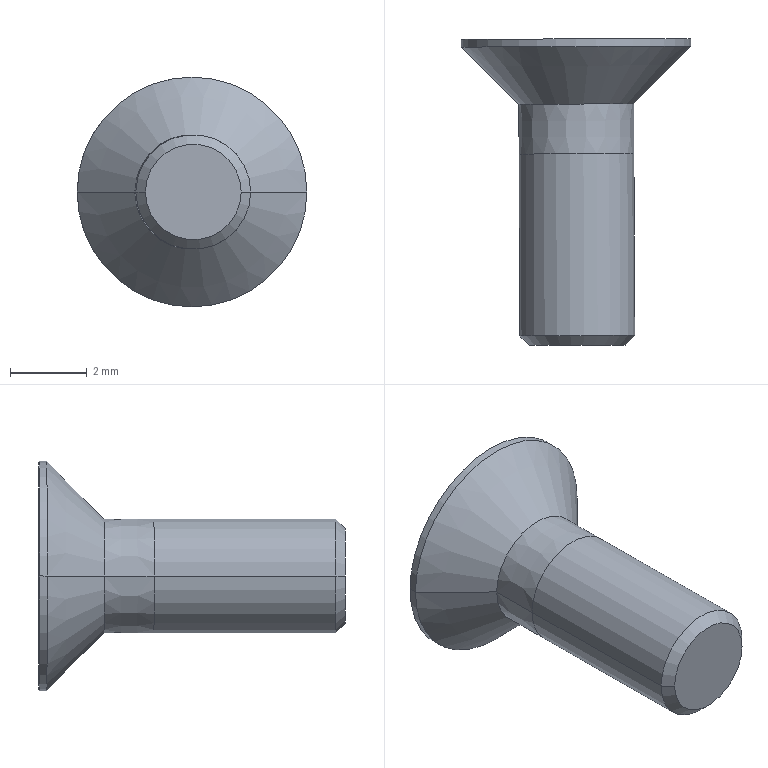Part | SolidWorks | features BaseBody 1 | 1 solid | 19 faces | box 6.001 x 8.018 x 6 mm | volume 70.49 mm3 | plane 9 | cone 6 | cylinder 4 | commonest cylinder face diameters 3 x2 6 x2
STEP:
#1=CARTESIAN_POINT('',(644.486,66.545,-56.15));
#2=VERTEX_POINT('',#1);
#3=CARTESIAN_POINT('',(650.486,66.571,-56.15));
#4=VERTEX_POINT('',#3);
#5=CARTESIAN_POINT('',(647.486,66.558,-56.15));
#6=DIRECTION('',(-0.004352,1.,0.000000003));
#7=DIRECTION('',(1.,0.004352,0.));
#8=AXIS2_PLACEMENT_3D('',#5,#6,#7);
#9=CIRCLE('',#8,3.);
#10=EDGE_CURVE('',#2,#4,#9,.T.);
#11=ORIENTED_EDGE('',*,*,#10,.F.);
#12=CARTESIAN_POINT('',(644.487,66.345,-56.15));
#13=VERTEX_POINT('',#12);
#14=CARTESIAN_POINT('',(644.487,66.445,-56.15));
#15=DIRECTION('',(0.004352,-1.,-0.000000003));
#16=VECTOR('',#15,1000.);
#17=LINE('',#14,#16);
#18=EDGE_CURVE('',#2,#13,#17,.T.);
#19=ORIENTED_EDGE('',*,*,#18,.T.);
#20=CARTESIAN_POINT('',(650.487,66.371,-56.15));
#21=VERTEX_POINT('',#20);
#22=CARTESIAN_POINT('',(647.487,66.358,-56.15));
#23=DIRECTION('',(-0.004352,1.,0.000000003));
#24=DIRECTION('',(1.,0.004352,0.));
#25=AXIS2_PLACEMENT_3D('',#22,#23,#24);
#26=CIRCLE('',#25,3.);
#27=EDGE_CURVE('',#13,#21,#26,.T.);
#28=ORIENTED_EDGE('',*,*,#27,.T.);
#29=CARTESIAN_POINT('',(650.487,66.471,-56.15));
#30=DIRECTION('',(0.004352,-1.,-0.000000003));
#31=VECTOR('',#30,1000.);
#32=LINE('',#29,#31);
#33=EDGE_CURVE('',#4,#21,#32,.T.);
#34=ORIENTED_EDGE('',*,*,#33,.F.);
#35=EDGE_LOOP('',(#11,#19,#28,#34));
#36=FACE_OUTER_BOUND('',#35,.T.);
#37=CARTESIAN_POINT('',(647.487,66.458,-56.15));
#38=DIRECTION('',(0.004352,-1.,-0.000000003));
#39=DIRECTION('',(1.,0.004352,0.));
#40=AXIS2_PLACEMENT_3D('',#37,#38,#39);
#41=CYLINDRICAL_SURFACE('',#40,3.);
#42=ADVANCED_FACE('',(#36),#41,.T.);
#43=CARTESIAN_POINT('',(645.994,64.852,-56.15));
#44=VERTEX_POINT('',#43);
#45=CARTESIAN_POINT('',(648.993,64.865,-56.15));
#46=VERTEX_POINT('',#45);
#47=CARTESIAN_POINT('',(647.494,64.858,-56.15));
#48=DIRECTION('',(-0.004352,1.,0.000000003));
#49=DIRECTION('',(-1.,-0.004352,0.));
#50=AXIS2_PLACEMENT_3D('',#47,#48,#49);
#51=CIRCLE('',#50,1.5);
#52=EDGE_CURVE('',#44,#46,#51,.T.);
#53=ORIENTED_EDGE('',*,*,#52,.T.);
#54=CARTESIAN_POINT('',(650.487,66.371,-56.15));
#55=DIRECTION('',(0.704,0.7102,0.000000002));
#56=VECTOR('',#55,1000.);
#57=LINE('',#54,#56);
#58=EDGE_CURVE('',#46,#21,#57,.T.);
#59=ORIENTED_EDGE('',*,*,#58,.T.);
#60=ORIENTED_EDGE('',*,*,#27,.F.);
#61=CARTESIAN_POINT('',(644.487,66.345,-56.15));
#62=DIRECTION('',(-0.7102,0.704,0.000000002));
#63=VECTOR('',#62,1000.);
#64=LINE('',#61,#63);
#65=EDGE_CURVE('',#44,#13,#64,.T.);
#66=ORIENTED_EDGE('',*,*,#65,.F.);
#67=EDGE_LOOP('',(#53,#59,#60,#66));
#68=FACE_OUTER_BOUND('',#67,.T.);
#69=CARTESIAN_POINT('',(647.487,66.358,-56.15));
#70=DIRECTION('',(-0.004352,1.,0.000000003));
#71=DIRECTION('',(-1.,-0.004352,0.));
#72=AXIS2_PLACEMENT_3D('',#69,#70,#71);
#73=CONICAL_SURFACE('',#72,3.,0.7854);
#74=ADVANCED_FACE('',(#68),#73,.T.);
#75=ORIENTED_EDGE('',*,*,#52,.F.);
#76=CARTESIAN_POINT('',(645.999,63.552,-56.15));
#77=VERTEX_POINT('',#76);
#78=CARTESIAN_POINT('',(645.999,63.552,-56.15));
#79=DIRECTION('',(0.004102,-1.,-0.000000003));
#80=VECTOR('',#79,1000.);
#81=LINE('',#78,#80);
#82=EDGE_CURVE('',#44,#77,#81,.T.);
#83=ORIENTED_EDGE('',*,*,#82,.T.);
#84=CARTESIAN_POINT('',(648.999,63.565,-56.15));
#85=VERTEX_POINT('',#84);
#86=CARTESIAN_POINT('',(647.499,63.558,-56.15));
#87=DIRECTION('',(-0.004352,1.,0.000000003));
#88=DIRECTION('',(-1.,-0.004352,0.000000001));
#89=AXIS2_PLACEMENT_3D('',#86,#87,#88);
#90=CIRCLE('',#89,1.5);
#91=EDGE_CURVE('',#77,#85,#90,.T.);
#92=ORIENTED_EDGE('',*,*,#91,.T.);
#93=CARTESIAN_POINT('',(648.999,63.565,-56.15));
#94=DIRECTION('',(0.004602,-1.,-0.000000003));
#95=VECTOR('',#94,1000.);
#96=LINE('',#93,#95);
#97=EDGE_CURVE('',#46,#85,#96,.T.);
#98=ORIENTED_EDGE('',*,*,#97,.F.);
#99=EDGE_LOOP('',(#75,#83,#92,#98));
#100=FACE_OUTER_BOUND('',#99,.T.);
#101=CARTESIAN_POINT('',(647.499,63.558,-56.15));
#102=DIRECTION('',(0.004352,-1.,-0.000000003));
#103=DIRECTION('',(1.,0.004352,0.));
#104=AXIS2_PLACEMENT_3D('',#101,#102,#103);
#105=CONICAL_SURFACE('',#104,1.5,0.00025);
#106=ADVANCED_FACE('',(#100),#105,.T.);
#107=ORIENTED_EDGE('',*,*,#91,.F.);
#108=CARTESIAN_POINT('',(646.02,58.802,-56.15));
#109=VERTEX_POINT('',#108);
#110=CARTESIAN_POINT('',(646.01,61.177,-56.15));
#111=DIRECTION('',(0.004352,-1.,-0.000000003));
#112=VECTOR('',#111,1000.);
#113=LINE('',#110,#112);
#114=EDGE_CURVE('',#77,#109,#113,.T.);
#115=ORIENTED_EDGE('',*,*,#114,.T.);
#116=CARTESIAN_POINT('',(649.02,58.815,-56.15));
#117=VERTEX_POINT('',#116);
#118=CARTESIAN_POINT('',(647.52,58.809,-56.15));
#119=DIRECTION('',(-0.004352,1.,0.000000003));
#120=DIRECTION('',(1.,0.004352,0.));
#121=AXIS2_PLACEMENT_3D('',#118,#119,#120);
#122=CIRCLE('',#121,1.5);
#123=EDGE_CURVE('',#109,#117,#122,.T.);
#124=ORIENTED_EDGE('',*,*,#123,.T.);
#125=CARTESIAN_POINT('',(649.01,61.19,-56.15));
#126=DIRECTION('',(0.004352,-1.,-0.000000003));
#127=VECTOR('',#126,1000.);
#128=LINE('',#125,#127);
#129=EDGE_CURVE('',#85,#117,#128,.T.);
#130=ORIENTED_EDGE('',*,*,#129,.F.);
#131=EDGE_LOOP('',(#107,#115,#124,#130));
#132=FACE_OUTER_BOUND('',#131,.T.);
#133=CARTESIAN_POINT('',(647.51,61.183,-56.15));
#134=DIRECTION('',(0.004352,-1.,-0.000000003));
#135=DIRECTION('',(1.,0.004352,0.));
#136=AXIS2_PLACEMENT_3D('',#133,#134,#135);
#137=CYLINDRICAL_SURFACE('',#136,1.5);
#138=ADVANCED_FACE('',(#132),#137,.T.);
#139=CARTESIAN_POINT('',(646.271,58.553,-56.15));
#140=VERTEX_POINT('',#139);
#141=CARTESIAN_POINT('',(648.771,58.564,-56.15));
#142=VERTEX_POINT('',#141);
#143=CARTESIAN_POINT('',(647.521,58.559,-56.15));
#144=DIRECTION('',(-0.004352,1.,0.000000003));
#145=DIRECTION('',(-1.,-0.004352,0.));
#146=AXIS2_PLACEMENT_3D('',#143,#144,#145);
#147=CIRCLE('',#146,1.25);
#148=EDGE_CURVE('',#140,#142,#147,.T.);
#149=ORIENTED_EDGE('',*,*,#148,.T.);
#150=CARTESIAN_POINT('',(649.02,58.815,-56.15));
#151=DIRECTION('',(0.704,0.7102,0.000000002));
#152=VECTOR('',#151,1000.);
#153=LINE('',#150,#152);
#154=EDGE_CURVE('',#142,#117,#153,.T.);
#155=ORIENTED_EDGE('',*,*,#154,.T.);
#156=ORIENTED_EDGE('',*,*,#123,.F.);
#157=CARTESIAN_POINT('',(646.02,58.802,-56.15));
#158=DIRECTION('',(-0.7102,0.704,0.000000002));
#159=VECTOR('',#158,1000.);
#160=LINE('',#157,#159);
#161=EDGE_CURVE('',#140,#109,#160,.T.);
#162=ORIENTED_EDGE('',*,*,#161,.F.);
#163=EDGE_LOOP('',(#149,#155,#156,#162));
#164=FACE_OUTER_BOUND('',#163,.T.);
#165=CARTESIAN_POINT('',(647.52,58.809,-56.15));
#166=DIRECTION('',(-0.004352,1.,0.000000003));
#167=DIRECTION('',(-1.,-0.004352,0.));
#168=AXIS2_PLACEMENT_3D('',#165,#166,#167);
#169=CONICAL_SURFACE('',#168,1.5,0.7854);
#170=ADVANCED_FACE('',(#164),#169,.T.);
#171=CARTESIAN_POINT('',(647.486,66.558,-56.15));
#172=DIRECTION('',(-0.004352,1.,0.000000003));
#173=DIRECTION('',(1.,0.004352,0.));
#174=AXIS2_PLACEMENT_3D('',#171,#172,#173);
#175=CIRCLE('',#174,3.);
#176=EDGE_CURVE('',#4,#2,#175,.T.);
#177=ORIENTED_EDGE('',*,*,#176,.T.);
#178=ORIENTED_EDGE('',*,*,#10,.T.);
#179=EDGE_LOOP('',(#177,#178));
#180=FACE_OUTER_BOUND('',#179,.T.);
#181=CARTESIAN_POINT('',(648.064,66.561,-57.15));
#182=VERTEX_POINT('',#181);
#183=CARTESIAN_POINT('',(648.641,66.563,-56.15));
#184=VERTEX_POINT('',#183);
#185=CARTESIAN_POINT('',(648.064,66.561,-57.15));
#186=DIRECTION('',(0.5,0.002176,0.866));
#187=VECTOR('',#186,1000.);
#188=LINE('',#185,#187);
#189=EDGE_CURVE('',#182,#184,#188,.T.);
#190=ORIENTED_EDGE('',*,*,#189,.T.);
#191=CARTESIAN_POINT('',(648.064,66.561,-55.15));
#192=VERTEX_POINT('',#191);
#193=CARTESIAN_POINT('',(648.641,66.563,-56.15));
#194=DIRECTION('',(-0.5,-0.002176,0.866));
#195=VECTOR('',#194,1000.);
#196=LINE('',#193,#195);
#197=EDGE_CURVE('',#184,#192,#196,.T.);
#198=ORIENTED_EDGE('',*,*,#197,.T.);
#199=CARTESIAN_POINT('',(646.909,66.556,-55.15));
#200=VERTEX_POINT('',#199);
#201=CARTESIAN_POINT('',(646.737,66.555,-55.15));
#202=DIRECTION('',(-1.,-0.004352,0.));
#203=VECTOR('',#202,1000.);
#204=LINE('',#201,#203);
#205=EDGE_CURVE('',#192,#200,#204,.T.);
#206=ORIENTED_EDGE('',*,*,#205,.T.);
#207=CARTESIAN_POINT('',(646.332,66.553,-56.15));
#208=VERTEX_POINT('',#207);
#209=CARTESIAN_POINT('',(646.909,66.556,-55.15));
#210=DIRECTION('',(-0.5,-0.002176,-0.866));
#211=VECTOR('',#210,1000.);
#212=LINE('',#209,#211);
#213=EDGE_CURVE('',#200,#208,#212,.T.);
#214=ORIENTED_EDGE('',*,*,#213,.T.);
#215=CARTESIAN_POINT('',(646.909,66.556,-57.15));
#216=VERTEX_POINT('',#215);
#217=CARTESIAN_POINT('',(646.332,66.553,-56.15));
#218=DIRECTION('',(0.5,0.002176,-0.866));
#219=VECTOR('',#218,1000.);
#220=LINE('',#217,#219);
#221=EDGE_CURVE('',#208,#216,#220,.T.);
#222=ORIENTED_EDGE('',*,*,#221,.T.);
#223=CARTESIAN_POINT('',(646.737,66.555,-57.15));
#224=DIRECTION('',(1.,0.004352,0.));
#225=VECTOR('',#224,1000.);
#226=LINE('',#223,#225);
#227=EDGE_CURVE('',#216,#182,#226,.T.);
#228=ORIENTED_EDGE('',*,*,#227,.T.);
#229=EDGE_LOOP('',(#190,#198,#206,#214,#222,#228));
#230=FACE_BOUND('',#229,.T.);
#231=CARTESIAN_POINT('',(646.737,66.555,-56.15));
#232=DIRECTION('',(-0.004352,1.,0.000000003));
#233=DIRECTION('',(-1.,-0.004352,0.));
#234=AXIS2_PLACEMENT_3D('',#231,#232,#233);
#235=PLANE('',#234);
#236=ADVANCED_FACE('',(#180,#230),#235,.T.);
#237=ORIENTED_EDGE('',*,*,#18,.F.);
#238=ORIENTED_EDGE('',*,*,#176,.F.);
#239=ORIENTED_EDGE('',*,*,#33,.T.);
#240=CARTESIAN_POINT('',(647.487,66.358,-56.15));
#241=DIRECTION('',(-0.004352,1.,0.000000003));
#242=DIRECTION('',(1.,0.004352,0.));
#243=AXIS2_PLACEMENT_3D('',#240,#241,#242);
#244=CIRCLE('',#243,3.);
#245=EDGE_CURVE('',#21,#13,#244,.T.);
#246=ORIENTED_EDGE('',*,*,#245,.T.);
#247=EDGE_LOOP('',(#237,#238,#239,#246));
#248=FACE_OUTER_BOUND('',#247,.T.);
#249=CARTESIAN_POINT('',(647.487,66.458,-56.15));
#250=DIRECTION('',(0.004352,-1.,-0.000000003));
#251=DIRECTION('',(1.,0.004352,0.));
#252=AXIS2_PLACEMENT_3D('',#249,#250,#251);
#253=CYLINDRICAL_SURFACE('',#252,3.);
#254=ADVANCED_FACE('',(#248),#253,.T.);
#255=CARTESIAN_POINT('',(648.069,65.361,-55.15));
#256=VERTEX_POINT('',#255);
#257=CARTESIAN_POINT('',(648.064,66.561,-55.15));
#258=DIRECTION('',(0.004352,-1.,-0.000000003));
#259=VECTOR('',#258,1000.);
#260=LINE('',#257,#259);
#261=EDGE_CURVE('',#192,#256,#260,.T.);
#262=ORIENTED_EDGE('',*,*,#261,.F.);
#263=ORIENTED_EDGE('',*,*,#197,.F.);
#264=CARTESIAN_POINT('',(648.646,65.363,-56.15));
#265=VERTEX_POINT('',#264);
#266=CARTESIAN_POINT('',(648.646,65.363,-56.15));
#267=DIRECTION('',(-0.004352,1.,0.000000003));
#268=VECTOR('',#267,1000.);
#269=LINE('',#266,#268);
#270=EDGE_CURVE('',#265,#184,#269,.T.);
#271=ORIENTED_EDGE('',*,*,#270,.F.);
#272=CARTESIAN_POINT('',(648.069,65.361,-55.15));
#273=DIRECTION('',(0.5,0.002176,-0.866));
#274=VECTOR('',#273,1000.);
#275=LINE('',#272,#274);
#276=EDGE_CURVE('',#256,#265,#275,.T.);
#277=ORIENTED_EDGE('',*,*,#276,.F.);
#278=EDGE_LOOP('',(#262,#263,#271,#277));
#279=FACE_OUTER_BOUND('',#278,.T.);
#280=CARTESIAN_POINT('',(648.064,66.561,-55.15));
#281=DIRECTION('',(0.866,0.003769,0.5));
#282=DIRECTION('',(0.5,0.,-0.866));
#283=AXIS2_PLACEMENT_3D('',#280,#281,#282);
#284=PLANE('',#283);
#285=ADVANCED_FACE('',(#279),#284,.F.);
#286=ORIENTED_EDGE('',*,*,#270,.T.);
#287=ORIENTED_EDGE('',*,*,#189,.F.);
#288=CARTESIAN_POINT('',(648.069,65.361,-57.15));
#289=VERTEX_POINT('',#288);
#290=CARTESIAN_POINT('',(648.069,65.361,-57.15));
#291=DIRECTION('',(-0.004352,1.,0.000000003));
#292=VECTOR('',#291,1000.);
#293=LINE('',#290,#292);
#294=EDGE_CURVE('',#289,#182,#293,.T.);
#295=ORIENTED_EDGE('',*,*,#294,.F.);
#296=CARTESIAN_POINT('',(648.646,65.363,-56.15));
#297=DIRECTION('',(-0.5,-0.002176,-0.866));
#298=VECTOR('',#297,1000.);
#299=LINE('',#296,#298);
#300=EDGE_CURVE('',#265,#289,#299,.T.);
#301=ORIENTED_EDGE('',*,*,#300,.F.);
#302=EDGE_LOOP('',(#286,#287,#295,#301));
#303=FACE_OUTER_BOUND('',#302,.T.);
#304=CARTESIAN_POINT('',(648.641,66.563,-56.15));
#305=DIRECTION('',(0.866,0.003769,-0.5));
#306=DIRECTION('',(-0.5,0.,-0.866));
#307=AXIS2_PLACEMENT_3D('',#304,#305,#306);
#308=PLANE('',#307);
#309=ADVANCED_FACE('',(#303),#308,.F.);
#310=ORIENTED_EDGE('',*,*,#294,.T.);
#311=ORIENTED_EDGE('',*,*,#227,.F.);
#312=CARTESIAN_POINT('',(646.914,65.356,-57.15));
#313=VERTEX_POINT('',#312);
#314=CARTESIAN_POINT('',(646.914,65.356,-57.15));
#315=DIRECTION('',(-0.004352,1.,0.000000003));
#316=VECTOR('',#315,1000.);
#317=LINE('',#314,#316);
#318=EDGE_CURVE('',#313,#216,#317,.T.);
#319=ORIENTED_EDGE('',*,*,#318,.F.);
#320=CARTESIAN_POINT('',(648.069,65.361,-57.15));
#321=DIRECTION('',(-1.,-0.004352,0.000000001));
#322=VECTOR('',#321,1000.);
#323=LINE('',#320,#322);
#324=EDGE_CURVE('',#289,#313,#323,.T.);
#325=ORIENTED_EDGE('',*,*,#324,.F.);
#326=EDGE_LOOP('',(#310,#311,#319,#325));
#327=FACE_OUTER_BOUND('',#326,.T.);
#328=CARTESIAN_POINT('',(648.064,66.561,-57.15));
#329=DIRECTION('',(-0.000000001,0.000000003,-1.));
#330=DIRECTION('',(0.,1.,0.000000003));
#331=AXIS2_PLACEMENT_3D('',#328,#329,#330);
#332=PLANE('',#331);
#333=ADVANCED_FACE('',(#327),#332,.F.);
#334=ORIENTED_EDGE('',*,*,#318,.T.);
#335=ORIENTED_EDGE('',*,*,#221,.F.);
#336=CARTESIAN_POINT('',(646.337,65.353,-56.15));
#337=VERTEX_POINT('',#336);
#338=CARTESIAN_POINT('',(646.337,65.353,-56.15));
#339=DIRECTION('',(-0.004352,1.,0.000000003));
#340=VECTOR('',#339,1000.);
#341=LINE('',#338,#340);
#342=EDGE_CURVE('',#337,#208,#341,.T.);
#343=ORIENTED_EDGE('',*,*,#342,.F.);
#344=CARTESIAN_POINT('',(646.914,65.356,-57.15));
#345=DIRECTION('',(-0.5,-0.002176,0.866));
#346=VECTOR('',#345,1000.);
#347=LINE('',#344,#346);
#348=EDGE_CURVE('',#313,#337,#347,.T.);
#349=ORIENTED_EDGE('',*,*,#348,.F.);
#350=EDGE_LOOP('',(#334,#335,#343,#349));
#351=FACE_OUTER_BOUND('',#350,.T.);
#352=CARTESIAN_POINT('',(646.909,66.556,-57.15));
#353=DIRECTION('',(-0.866,-0.003769,-0.5));
#354=DIRECTION('',(-0.5,0.,0.866));
#355=AXIS2_PLACEMENT_3D('',#352,#353,#354);
#356=PLANE('',#355);
#357=ADVANCED_FACE('',(#351),#356,.F.);
#358=ORIENTED_EDGE('',*,*,#342,.T.);
#359=ORIENTED_EDGE('',*,*,#213,.F.);
#360=CARTESIAN_POINT('',(646.914,65.356,-55.15));
#361=VERTEX_POINT('',#360);
#362=CARTESIAN_POINT('',(646.914,65.356,-55.15));
#363=DIRECTION('',(-0.004352,1.,0.000000003));
#364=VECTOR('',#363,1000.);
#365=LINE('',#362,#364);
#366=EDGE_CURVE('',#361,#200,#365,.T.);
#367=ORIENTED_EDGE('',*,*,#366,.F.);
#368=CARTESIAN_POINT('',(646.337,65.353,-56.15));
#369=DIRECTION('',(0.5,0.002176,0.866));
#370=VECTOR('',#369,1000.);
#371=LINE('',#368,#370);
#372=EDGE_CURVE('',#337,#361,#371,.T.);
#373=ORIENTED_EDGE('',*,*,#372,.F.);
#374=EDGE_LOOP('',(#358,#359,#367,#373));
#375=FACE_OUTER_BOUND('',#374,.T.);
#376=CARTESIAN_POINT('',(646.332,66.553,-56.15));
#377=DIRECTION('',(-0.866,-0.003769,0.5));
#378=DIRECTION('',(0.5,0.,0.866));
#379=AXIS2_PLACEMENT_3D('',#376,#377,#378);
#380=PLANE('',#379);
#381=ADVANCED_FACE('',(#375),#380,.F.);
#382=ORIENTED_EDGE('',*,*,#366,.T.);
#383=ORIENTED_EDGE('',*,*,#205,.F.);
#384=ORIENTED_EDGE('',*,*,#261,.T.);
#385=CARTESIAN_POINT('',(646.914,65.356,-55.15));
#386=DIRECTION('',(1.,0.004352,-0.000000001));
#387=VECTOR('',#386,1000.);
#388=LINE('',#385,#387);
#389=EDGE_CURVE('',#361,#256,#388,.T.);
#390=ORIENTED_EDGE('',*,*,#389,.F.);
#391=EDGE_LOOP('',(#382,#383,#384,#390));
#392=FACE_OUTER_BOUND('',#391,.T.);
#393=CARTESIAN_POINT('',(646.909,66.556,-55.15));
#394=DIRECTION('',(0.000000001,-0.000000003,1.));
#395=DIRECTION('',(0.,-1.,-0.000000003));
#396=AXIS2_PLACEMENT_3D('',#393,#394,#395);
#397=PLANE('',#396);
#398=ADVANCED_FACE('',(#392),#397,.F.);
#399=ORIENTED_EDGE('',*,*,#58,.F.);
#400=CARTESIAN_POINT('',(647.494,64.858,-56.15));
#401=DIRECTION('',(-0.004352,1.,0.000000003));
#402=DIRECTION('',(-1.,-0.004352,0.));
#403=AXIS2_PLACEMENT_3D('',#400,#401,#402);
#404=CIRCLE('',#403,1.5);
#405=EDGE_CURVE('',#46,#44,#404,.T.);
#406=ORIENTED_EDGE('',*,*,#405,.T.);
#407=ORIENTED_EDGE('',*,*,#65,.T.);
#408=ORIENTED_EDGE('',*,*,#245,.F.);
#409=EDGE_LOOP('',(#399,#406,#407,#408));
#410=FACE_OUTER_BOUND('',#409,.T.);
#411=CARTESIAN_POINT('',(647.487,66.358,-56.15));
#412=DIRECTION('',(-0.004352,1.,0.000000003));
#413=DIRECTION('',(-1.,-0.004352,0.));
#414=AXIS2_PLACEMENT_3D('',#411,#412,#413);
#415=CONICAL_SURFACE('',#414,3.,0.7854);
#416=ADVANCED_FACE('',(#410),#415,.T.);
#417=ORIENTED_EDGE('',*,*,#348,.T.);
#418=ORIENTED_EDGE('',*,*,#372,.T.);
#419=ORIENTED_EDGE('',*,*,#389,.T.);
#420=ORIENTED_EDGE('',*,*,#276,.T.);
#421=ORIENTED_EDGE('',*,*,#300,.T.);
#422=ORIENTED_EDGE('',*,*,#324,.T.);
#423=EDGE_LOOP('',(#417,#418,#419,#420,#421,#422));
#424=FACE_OUTER_BOUND('',#423,.T.);
#425=CARTESIAN_POINT('',(647.492,65.358,-56.15));
#426=DIRECTION('',(-0.004352,1.,0.000000003));
#427=DIRECTION('',(-1.,-0.004352,0.));
#428=AXIS2_PLACEMENT_3D('',#425,#426,#427);
#429=PLANE('',#428);
#430=ADVANCED_FACE('',(#424),#429,.T.);
#431=ORIENTED_EDGE('',*,*,#82,.F.);
#432=ORIENTED_EDGE('',*,*,#405,.F.);
#433=ORIENTED_EDGE('',*,*,#97,.T.);
#434=CARTESIAN_POINT('',(647.499,63.558,-56.15));
#435=DIRECTION('',(-0.004352,1.,0.000000003));
#436=DIRECTION('',(-1.,-0.004352,0.000000001));
#437=AXIS2_PLACEMENT_3D('',#434,#435,#436);
#438=CIRCLE('',#437,1.5);
#439=EDGE_CURVE('',#85,#77,#438,.T.);
#440=ORIENTED_EDGE('',*,*,#439,.T.);
#441=EDGE_LOOP('',(#431,#432,#433,#440));
#442=FACE_OUTER_BOUND('',#441,.T.);
#443=CARTESIAN_POINT('',(647.499,63.558,-56.15));
#444=DIRECTION('',(0.004352,-1.,-0.000000003));
#445=DIRECTION('',(1.,0.004352,0.));
#446=AXIS2_PLACEMENT_3D('',#443,#444,#445);
#447=CONICAL_SURFACE('',#446,1.5,0.00025);
#448=ADVANCED_FACE('',(#442),#447,.T.);
#449=ORIENTED_EDGE('',*,*,#114,.F.);
#450=ORIENTED_EDGE('',*,*,#439,.F.);
#451=ORIENTED_EDGE('',*,*,#129,.T.);
#452=CARTESIAN_POINT('',(647.52,58.809,-56.15));
#453=DIRECTION('',(-0.004352,1.,0.000000003));
#454=DIRECTION('',(1.,0.004352,0.));
#455=AXIS2_PLACEMENT_3D('',#452,#453,#454);
#456=CIRCLE('',#455,1.5);
#457=EDGE_CURVE('',#117,#109,#456,.T.);
#458=ORIENTED_EDGE('',*,*,#457,.T.);
#459=EDGE_LOOP('',(#449,#450,#451,#458));
#460=FACE_OUTER_BOUND('',#459,.T.);
#461=CARTESIAN_POINT('',(647.51,61.183,-56.15));
#462=DIRECTION('',(0.004352,-1.,-0.000000003));
#463=DIRECTION('',(1.,0.004352,0.));
#464=AXIS2_PLACEMENT_3D('',#461,#462,#463);
#465=CYLINDRICAL_SURFACE('',#464,1.5);
#466=ADVANCED_FACE('',(#460),#465,.T.);
#467=ORIENTED_EDGE('',*,*,#154,.F.);
#468=CARTESIAN_POINT('',(647.521,58.559,-56.15));
#469=DIRECTION('',(-0.004352,1.,0.000000003));
#470=DIRECTION('',(-1.,-0.004352,0.));
#471=AXIS2_PLACEMENT_3D('',#468,#469,#470);
#472=CIRCLE('',#471,1.25);
#473=EDGE_CURVE('',#142,#140,#472,.T.);
#474=ORIENTED_EDGE('',*,*,#473,.T.);
#475=ORIENTED_EDGE('',*,*,#161,.T.);
#476=ORIENTED_EDGE('',*,*,#457,.F.);
#477=EDGE_LOOP('',(#467,#474,#475,#476));
#478=FACE_OUTER_BOUND('',#477,.T.);
#479=CARTESIAN_POINT('',(647.52,58.809,-56.15));
#480=DIRECTION('',(-0.004352,1.,0.000000003));
#481=DIRECTION('',(-1.,-0.004352,0.));
#482=AXIS2_PLACEMENT_3D('',#479,#480,#481);
#483=CONICAL_SURFACE('',#482,1.5,0.7854);
#484=ADVANCED_FACE('',(#478),#483,.T.);
#485=ORIENTED_EDGE('',*,*,#148,.F.);
#486=ORIENTED_EDGE('',*,*,#473,.F.);
#487=EDGE_LOOP('',(#485,#486));
#488=FACE_OUTER_BOUND('',#487,.T.);
#489=CARTESIAN_POINT('',(646.896,58.556,-56.15));
#490=DIRECTION('',(0.004352,-1.,-0.000000003));
#491=DIRECTION('',(1.,0.004352,0.));
#492=AXIS2_PLACEMENT_3D('',#489,#490,#491);
#493=PLANE('',#492);
#494=ADVANCED_FACE('',(#488),#493,.T.);
#495=CLOSED_SHELL('',(#42,#74,#106,#138,#170,#236,#254,#285,#309,#333,#357,#381,#398,#416,#430,#448,#466,#484,#494));
#496=MANIFOLD_SOLID_BREP('',#495);
#497=CARTESIAN_POINT('',(0.,0.,0.));
#498=DIRECTION('',(0.,0.,1.));
#499=DIRECTION('',(1.,0.,0.));
#500=AXIS2_PLACEMENT_3D('',#497,#498,#499);
#501=(LENGTH_UNIT()NAMED_UNIT(*)SI_UNIT(.MILLI.,.METRE.));
#502=UNCERTAINTY_MEASURE_WITH_UNIT(LENGTH_MEASURE(0.00001),#501,'','');
#503=(NAMED_UNIT(*)PLANE_ANGLE_UNIT()SI_UNIT($,.RADIAN.));
#504=(NAMED_UNIT(*)SI_UNIT($,.STERADIAN.)SOLID_ANGLE_UNIT());
#505=(GEOMETRIC_REPRESENTATION_CONTEXT(3)GLOBAL_UNCERTAINTY_ASSIGNED_CONTEXT((#502))GLOBAL_UNIT_ASSIGNED_CONTEXT((#501,#503,#504))REPRESENTATION_CONTEXT('',''));
#506=ADVANCED_BREP_SHAPE_REPRESENTATION('',(#496,#500),#505);